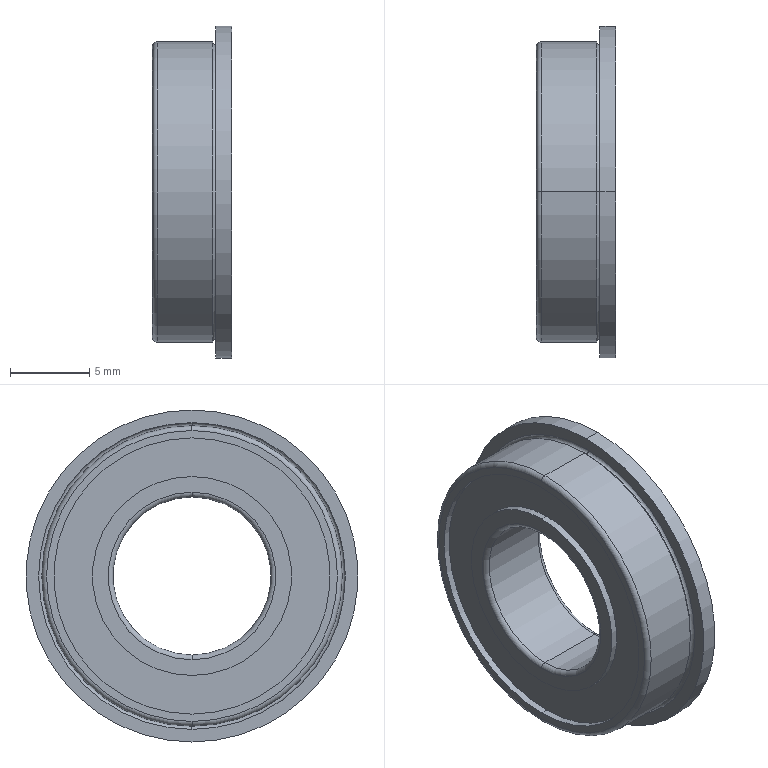Part | NX | features BREP 1 | 1 solid | 31 faces | box 5 x 21 x 21 mm | volume 978.232 mm3 | cylinder 14 | torus 10 | plane 7 | commonest cylinder face diameters 12.58 x4 17.47 x4 10 x2 19 x2 21 x2
STEP:
#1=CARTESIAN_POINT('',(0.,0.,9.3));
#2=VERTEX_POINT('',#1);
#3=CARTESIAN_POINT('',(-0.2,0.,9.5));
#4=VERTEX_POINT('',#3);
#5=CARTESIAN_POINT('',(0.,0.,9.5));
#6=DIRECTION('',(0.,-1.,0.));
#7=DIRECTION('',(0.,0.,-1.));
#8=AXIS2_PLACEMENT_3D('',#5,#6,#7);
#9=CIRCLE('',#8,0.2);
#10=EDGE_CURVE('',#2,#4,#9,.F.);
#11=ORIENTED_EDGE('',*,*,#10,.F.);
#12=CARTESIAN_POINT('',(0.,0.,-9.3));
#13=VERTEX_POINT('',#12);
#14=CARTESIAN_POINT('',(0.,0.,0.));
#15=DIRECTION('',(-1.,0.,0.));
#16=DIRECTION('',(0.,0.,1.));
#17=AXIS2_PLACEMENT_3D('',#14,#15,#16);
#18=CIRCLE('',#17,9.3);
#19=EDGE_CURVE('',#2,#13,#18,.T.);
#20=ORIENTED_EDGE('',*,*,#19,.T.);
#21=CARTESIAN_POINT('',(-0.2,0.,-9.5));
#22=VERTEX_POINT('',#21);
#23=CARTESIAN_POINT('',(0.,0.,-9.5));
#24=DIRECTION('',(0.,1.,0.));
#25=DIRECTION('',(0.,0.,1.));
#26=AXIS2_PLACEMENT_3D('',#23,#24,#25);
#27=CIRCLE('',#26,0.2);
#28=EDGE_CURVE('',#13,#22,#27,.F.);
#29=ORIENTED_EDGE('',*,*,#28,.T.);
#30=CARTESIAN_POINT('',(-0.2,0.,0.));
#31=DIRECTION('',(-1.,0.,0.));
#32=DIRECTION('',(0.,0.,1.));
#33=AXIS2_PLACEMENT_3D('',#30,#31,#32);
#34=CIRCLE('',#33,9.5);
#35=EDGE_CURVE('',#4,#22,#34,.T.);
#36=ORIENTED_EDGE('',*,*,#35,.F.);
#37=EDGE_LOOP('',(#11,#20,#29,#36));
#38=FACE_BOUND('',#37,.T.);
#39=CARTESIAN_POINT('',(0.,0.,0.));
#40=DIRECTION('',(-1.,0.,0.));
#41=DIRECTION('',(0.,0.,-1.));
#42=AXIS2_PLACEMENT_3D('',#39,#40,#41);
#43=TOROIDAL_SURFACE('',#42,9.5,0.2);
#44=ADVANCED_FACE('',(#38),#43,.F.);
#45=ORIENTED_EDGE('',*,*,#28,.F.);
#46=CARTESIAN_POINT('',(0.,0.,0.));
#47=DIRECTION('',(-1.,0.,0.));
#48=DIRECTION('',(0.,0.,1.));
#49=AXIS2_PLACEMENT_3D('',#46,#47,#48);
#50=CIRCLE('',#49,9.3);
#51=EDGE_CURVE('',#13,#2,#50,.T.);
#52=ORIENTED_EDGE('',*,*,#51,.T.);
#53=ORIENTED_EDGE('',*,*,#10,.T.);
#54=CARTESIAN_POINT('',(-0.2,0.,0.));
#55=DIRECTION('',(-1.,0.,0.));
#56=DIRECTION('',(0.,0.,1.));
#57=AXIS2_PLACEMENT_3D('',#54,#55,#56);
#58=CIRCLE('',#57,9.5);
#59=EDGE_CURVE('',#22,#4,#58,.T.);
#60=ORIENTED_EDGE('',*,*,#59,.F.);
#61=EDGE_LOOP('',(#45,#52,#53,#60));
#62=FACE_BOUND('',#61,.T.);
#63=CARTESIAN_POINT('',(0.,0.,0.));
#64=DIRECTION('',(-1.,0.,0.));
#65=DIRECTION('',(0.,0.,-1.));
#66=AXIS2_PLACEMENT_3D('',#63,#64,#65);
#67=TOROIDAL_SURFACE('',#66,9.5,0.2);
#68=ADVANCED_FACE('',(#62),#67,.F.);
#69=CARTESIAN_POINT('',(-4.,0.,9.2));
#70=VERTEX_POINT('',#69);
#71=CARTESIAN_POINT('',(-4.,0.,-9.2));
#72=VERTEX_POINT('',#71);
#73=CARTESIAN_POINT('',(-4.,0.,0.));
#74=DIRECTION('',(-1.,0.,0.));
#75=DIRECTION('',(0.,0.,-1.));
#76=AXIS2_PLACEMENT_3D('',#73,#74,#75);
#77=CIRCLE('',#76,9.2);
#78=EDGE_CURVE('',#70,#72,#77,.T.);
#79=ORIENTED_EDGE('',*,*,#78,.F.);
#80=CARTESIAN_POINT('',(-3.7,0.,9.5));
#81=VERTEX_POINT('',#80);
#82=CARTESIAN_POINT('',(-3.7,0.,9.2));
#83=DIRECTION('',(0.,1.,0.));
#84=DIRECTION('',(0.,0.,1.));
#85=AXIS2_PLACEMENT_3D('',#82,#83,#84);
#86=CIRCLE('',#85,0.3);
#87=EDGE_CURVE('',#81,#70,#86,.F.);
#88=ORIENTED_EDGE('',*,*,#87,.F.);
#89=CARTESIAN_POINT('',(-3.7,0.,-9.5));
#90=VERTEX_POINT('',#89);
#91=CARTESIAN_POINT('',(-3.7,0.,0.));
#92=DIRECTION('',(1.,0.,0.));
#93=DIRECTION('',(0.,0.,-1.));
#94=AXIS2_PLACEMENT_3D('',#91,#92,#93);
#95=CIRCLE('',#94,9.5);
#96=EDGE_CURVE('',#90,#81,#95,.T.);
#97=ORIENTED_EDGE('',*,*,#96,.F.);
#98=CARTESIAN_POINT('',(-3.7,0.,-9.2));
#99=DIRECTION('',(0.,-1.,0.));
#100=DIRECTION('',(0.,0.,-1.));
#101=AXIS2_PLACEMENT_3D('',#98,#99,#100);
#102=CIRCLE('',#101,0.3);
#103=EDGE_CURVE('',#90,#72,#102,.F.);
#104=ORIENTED_EDGE('',*,*,#103,.T.);
#105=EDGE_LOOP('',(#79,#88,#97,#104));
#106=FACE_BOUND('',#105,.T.);
#107=CARTESIAN_POINT('',(-3.7,0.,0.));
#108=DIRECTION('',(1.,0.,0.));
#109=DIRECTION('',(0.,0.,1.));
#110=AXIS2_PLACEMENT_3D('',#107,#108,#109);
#111=TOROIDAL_SURFACE('',#110,9.2,0.3);
#112=ADVANCED_FACE('',(#106),#111,.T.);
#113=CARTESIAN_POINT('',(-3.7,0.,5.));
#114=VERTEX_POINT('',#113);
#115=CARTESIAN_POINT('',(-3.7,0.,-5.));
#116=VERTEX_POINT('',#115);
#117=CARTESIAN_POINT('',(-3.7,0.,0.));
#118=DIRECTION('',(-1.,0.,0.));
#119=DIRECTION('',(0.,0.,-1.));
#120=AXIS2_PLACEMENT_3D('',#117,#118,#119);
#121=CIRCLE('',#120,5.);
#122=EDGE_CURVE('',#114,#116,#121,.T.);
#123=ORIENTED_EDGE('',*,*,#122,.F.);
#124=CARTESIAN_POINT('',(-4.,0.,5.3));
#125=VERTEX_POINT('',#124);
#126=CARTESIAN_POINT('',(-3.7,0.,5.3));
#127=DIRECTION('',(0.,1.,0.));
#128=DIRECTION('',(0.,0.,1.));
#129=AXIS2_PLACEMENT_3D('',#126,#127,#128);
#130=CIRCLE('',#129,0.3);
#131=EDGE_CURVE('',#125,#114,#130,.F.);
#132=ORIENTED_EDGE('',*,*,#131,.F.);
#133=CARTESIAN_POINT('',(-4.,0.,-5.3));
#134=VERTEX_POINT('',#133);
#135=CARTESIAN_POINT('',(-4.,0.,0.));
#136=DIRECTION('',(1.,0.,0.));
#137=DIRECTION('',(0.,0.,-1.));
#138=AXIS2_PLACEMENT_3D('',#135,#136,#137);
#139=CIRCLE('',#138,5.3);
#140=EDGE_CURVE('',#134,#125,#139,.T.);
#141=ORIENTED_EDGE('',*,*,#140,.F.);
#142=CARTESIAN_POINT('',(-3.7,0.,-5.3));
#143=DIRECTION('',(0.,-1.,0.));
#144=DIRECTION('',(0.,0.,-1.));
#145=AXIS2_PLACEMENT_3D('',#142,#143,#144);
#146=CIRCLE('',#145,0.3);
#147=EDGE_CURVE('',#134,#116,#146,.F.);
#148=ORIENTED_EDGE('',*,*,#147,.T.);
#149=EDGE_LOOP('',(#123,#132,#141,#148));
#150=FACE_BOUND('',#149,.T.);
#151=CARTESIAN_POINT('',(-3.7,0.,0.));
#152=DIRECTION('',(1.,0.,0.));
#153=DIRECTION('',(0.,0.,1.));
#154=AXIS2_PLACEMENT_3D('',#151,#152,#153);
#155=TOROIDAL_SURFACE('',#154,5.3,0.3);
#156=ADVANCED_FACE('',(#150),#155,.T.);
#157=CARTESIAN_POINT('',(0.7,0.,-5.));
#158=VERTEX_POINT('',#157);
#159=CARTESIAN_POINT('',(0.7,0.,5.));
#160=VERTEX_POINT('',#159);
#161=CARTESIAN_POINT('',(0.7,0.,0.));
#162=DIRECTION('',(1.,0.,0.));
#163=DIRECTION('',(0.,0.,1.));
#164=AXIS2_PLACEMENT_3D('',#161,#162,#163);
#165=CIRCLE('',#164,5.);
#166=EDGE_CURVE('',#158,#160,#165,.T.);
#167=ORIENTED_EDGE('',*,*,#166,.F.);
#168=CARTESIAN_POINT('',(1.,0.,-5.3));
#169=VERTEX_POINT('',#168);
#170=CARTESIAN_POINT('',(0.7,0.,-5.3));
#171=DIRECTION('',(0.,1.,0.));
#172=DIRECTION('',(0.,0.,1.));
#173=AXIS2_PLACEMENT_3D('',#170,#171,#172);
#174=CIRCLE('',#173,0.3);
#175=EDGE_CURVE('',#158,#169,#174,.T.);
#176=ORIENTED_EDGE('',*,*,#175,.T.);
#177=CARTESIAN_POINT('',(1.,0.,5.3));
#178=VERTEX_POINT('',#177);
#179=CARTESIAN_POINT('',(1.,0.,0.));
#180=DIRECTION('',(-1.,0.,0.));
#181=DIRECTION('',(0.,0.,1.));
#182=AXIS2_PLACEMENT_3D('',#179,#180,#181);
#183=CIRCLE('',#182,5.3);
#184=EDGE_CURVE('',#178,#169,#183,.T.);
#185=ORIENTED_EDGE('',*,*,#184,.F.);
#186=CARTESIAN_POINT('',(0.7,0.,5.3));
#187=DIRECTION('',(0.,-1.,0.));
#188=DIRECTION('',(0.,0.,-1.));
#189=AXIS2_PLACEMENT_3D('',#186,#187,#188);
#190=CIRCLE('',#189,0.3);
#191=EDGE_CURVE('',#160,#178,#190,.T.);
#192=ORIENTED_EDGE('',*,*,#191,.F.);
#193=EDGE_LOOP('',(#167,#176,#185,#192));
#194=FACE_BOUND('',#193,.T.);
#195=CARTESIAN_POINT('',(0.7,0.,0.));
#196=DIRECTION('',(-1.,0.,0.));
#197=DIRECTION('',(0.,0.,-1.));
#198=AXIS2_PLACEMENT_3D('',#195,#196,#197);
#199=TOROIDAL_SURFACE('',#198,5.3,0.3);
#200=ADVANCED_FACE('',(#194),#199,.T.);
#201=CARTESIAN_POINT('',(1.,0.,-8.735));
#202=VERTEX_POINT('',#201);
#203=CARTESIAN_POINT('',(1.,0.,8.735));
#204=VERTEX_POINT('',#203);
#205=CARTESIAN_POINT('',(1.,0.,0.));
#206=DIRECTION('',(-1.,0.,0.));
#207=DIRECTION('',(0.,0.,1.));
#208=AXIS2_PLACEMENT_3D('',#205,#206,#207);
#209=CIRCLE('',#208,8.735);
#210=EDGE_CURVE('',#202,#204,#209,.T.);
#211=ORIENTED_EDGE('',*,*,#210,.F.);
#212=CARTESIAN_POINT('',(0.56,0.,-8.735));
#213=VERTEX_POINT('',#212);
#214=CARTESIAN_POINT('',(-4.,0.,-8.735));
#215=DIRECTION('',(-1.,0.,0.));
#216=VECTOR('',#215,1000.);
#217=LINE('',#214,#216);
#218=EDGE_CURVE('',#202,#213,#217,.T.);
#219=ORIENTED_EDGE('',*,*,#218,.T.);
#220=CARTESIAN_POINT('',(0.56,0.,8.735));
#221=VERTEX_POINT('',#220);
#222=CARTESIAN_POINT('',(0.56,0.,0.));
#223=DIRECTION('',(-1.,0.,0.));
#224=DIRECTION('',(0.,0.,1.));
#225=AXIS2_PLACEMENT_3D('',#222,#223,#224);
#226=CIRCLE('',#225,8.735);
#227=EDGE_CURVE('',#213,#221,#226,.T.);
#228=ORIENTED_EDGE('',*,*,#227,.T.);
#229=CARTESIAN_POINT('',(-4.,0.,8.735));
#230=DIRECTION('',(-1.,0.,0.));
#231=VECTOR('',#230,1000.);
#232=LINE('',#229,#231);
#233=EDGE_CURVE('',#204,#221,#232,.T.);
#234=ORIENTED_EDGE('',*,*,#233,.F.);
#235=EDGE_LOOP('',(#211,#219,#228,#234));
#236=FACE_BOUND('',#235,.T.);
#237=CARTESIAN_POINT('',(-4.,0.,0.));
#238=DIRECTION('',(-1.,0.,0.));
#239=DIRECTION('',(0.,0.,-1.));
#240=AXIS2_PLACEMENT_3D('',#237,#238,#239);
#241=CYLINDRICAL_SURFACE('',#240,8.735);
#242=ADVANCED_FACE('',(#236),#241,.F.);
#243=CARTESIAN_POINT('',(1.,0.,6.29));
#244=VERTEX_POINT('',#243);
#245=CARTESIAN_POINT('',(1.,0.,-6.29));
#246=VERTEX_POINT('',#245);
#247=CARTESIAN_POINT('',(1.,0.,0.));
#248=DIRECTION('',(-1.,0.,0.));
#249=DIRECTION('',(0.,0.,1.));
#250=AXIS2_PLACEMENT_3D('',#247,#248,#249);
#251=CIRCLE('',#250,6.29);
#252=EDGE_CURVE('',#244,#246,#251,.T.);
#253=ORIENTED_EDGE('',*,*,#252,.T.);
#254=CARTESIAN_POINT('',(0.56,0.,-6.29));
#255=VERTEX_POINT('',#254);
#256=CARTESIAN_POINT('',(-4.,0.,-6.29));
#257=DIRECTION('',(-1.,0.,0.));
#258=VECTOR('',#257,1000.);
#259=LINE('',#256,#258);
#260=EDGE_CURVE('',#246,#255,#259,.T.);
#261=ORIENTED_EDGE('',*,*,#260,.T.);
#262=CARTESIAN_POINT('',(0.56,0.,6.29));
#263=VERTEX_POINT('',#262);
#264=CARTESIAN_POINT('',(0.56,0.,0.));
#265=DIRECTION('',(-1.,0.,0.));
#266=DIRECTION('',(0.,0.,1.));
#267=AXIS2_PLACEMENT_3D('',#264,#265,#266);
#268=CIRCLE('',#267,6.29);
#269=EDGE_CURVE('',#263,#255,#268,.T.);
#270=ORIENTED_EDGE('',*,*,#269,.F.);
#271=CARTESIAN_POINT('',(-4.,0.,6.29));
#272=DIRECTION('',(-1.,0.,0.));
#273=VECTOR('',#272,1000.);
#274=LINE('',#271,#273);
#275=EDGE_CURVE('',#244,#263,#274,.T.);
#276=ORIENTED_EDGE('',*,*,#275,.F.);
#277=EDGE_LOOP('',(#253,#261,#270,#276));
#278=FACE_BOUND('',#277,.T.);
#279=CARTESIAN_POINT('',(-4.,0.,0.));
#280=DIRECTION('',(-1.,0.,0.));
#281=DIRECTION('',(0.,0.,-1.));
#282=AXIS2_PLACEMENT_3D('',#279,#280,#281);
#283=CYLINDRICAL_SURFACE('',#282,6.29);
#284=ADVANCED_FACE('',(#278),#283,.T.);
#285=CARTESIAN_POINT('',(0.7,0.,0.));
#286=DIRECTION('',(1.,0.,0.));
#287=DIRECTION('',(0.,0.,1.));
#288=AXIS2_PLACEMENT_3D('',#285,#286,#287);
#289=CIRCLE('',#288,5.);
#290=EDGE_CURVE('',#160,#158,#289,.T.);
#291=ORIENTED_EDGE('',*,*,#290,.T.);
#292=CARTESIAN_POINT('',(-4.,0.,-5.));
#293=DIRECTION('',(-1.,0.,0.));
#294=VECTOR('',#293,1000.);
#295=LINE('',#292,#294);
#296=EDGE_CURVE('',#158,#116,#295,.T.);
#297=ORIENTED_EDGE('',*,*,#296,.T.);
#298=CARTESIAN_POINT('',(-3.7,0.,0.));
#299=DIRECTION('',(-1.,0.,0.));
#300=DIRECTION('',(0.,0.,-1.));
#301=AXIS2_PLACEMENT_3D('',#298,#299,#300);
#302=CIRCLE('',#301,5.);
#303=EDGE_CURVE('',#116,#114,#302,.T.);
#304=ORIENTED_EDGE('',*,*,#303,.T.);
#305=CARTESIAN_POINT('',(-4.,0.,5.));
#306=DIRECTION('',(-1.,0.,0.));
#307=VECTOR('',#306,1000.);
#308=LINE('',#305,#307);
#309=EDGE_CURVE('',#160,#114,#308,.T.);
#310=ORIENTED_EDGE('',*,*,#309,.F.);
#311=EDGE_LOOP('',(#291,#297,#304,#310));
#312=FACE_BOUND('',#311,.T.);
#313=CARTESIAN_POINT('',(-4.,0.,0.));
#314=DIRECTION('',(-1.,0.,0.));
#315=DIRECTION('',(0.,0.,-1.));
#316=AXIS2_PLACEMENT_3D('',#313,#314,#315);
#317=CYLINDRICAL_SURFACE('',#316,5.);
#318=ADVANCED_FACE('',(#312),#317,.F.);
#319=CARTESIAN_POINT('',(-3.56,0.,6.29));
#320=VERTEX_POINT('',#319);
#321=CARTESIAN_POINT('',(-3.56,0.,-6.29));
#322=VERTEX_POINT('',#321);
#323=CARTESIAN_POINT('',(-3.56,0.,0.));
#324=DIRECTION('',(-1.,0.,0.));
#325=DIRECTION('',(0.,0.,1.));
#326=AXIS2_PLACEMENT_3D('',#323,#324,#325);
#327=CIRCLE('',#326,6.29);
#328=EDGE_CURVE('',#320,#322,#327,.T.);
#329=ORIENTED_EDGE('',*,*,#328,.T.);
#330=CARTESIAN_POINT('',(-4.,0.,-6.29));
#331=VERTEX_POINT('',#330);
#332=CARTESIAN_POINT('',(-4.,0.,-6.29));
#333=DIRECTION('',(-1.,0.,0.));
#334=VECTOR('',#333,1000.);
#335=LINE('',#332,#334);
#336=EDGE_CURVE('',#322,#331,#335,.T.);
#337=ORIENTED_EDGE('',*,*,#336,.T.);
#338=CARTESIAN_POINT('',(-4.,0.,6.29));
#339=VERTEX_POINT('',#338);
#340=CARTESIAN_POINT('',(-4.,0.,0.));
#341=DIRECTION('',(-1.,0.,0.));
#342=DIRECTION('',(0.,0.,1.));
#343=AXIS2_PLACEMENT_3D('',#340,#341,#342);
#344=CIRCLE('',#343,6.29);
#345=EDGE_CURVE('',#339,#331,#344,.T.);
#346=ORIENTED_EDGE('',*,*,#345,.F.);
#347=CARTESIAN_POINT('',(-4.,0.,6.29));
#348=DIRECTION('',(-1.,0.,0.));
#349=VECTOR('',#348,1000.);
#350=LINE('',#347,#349);
#351=EDGE_CURVE('',#320,#339,#350,.T.);
#352=ORIENTED_EDGE('',*,*,#351,.F.);
#353=EDGE_LOOP('',(#329,#337,#346,#352));
#354=FACE_BOUND('',#353,.T.);
#355=CARTESIAN_POINT('',(-4.,0.,0.));
#356=DIRECTION('',(-1.,0.,0.));
#357=DIRECTION('',(0.,0.,-1.));
#358=AXIS2_PLACEMENT_3D('',#355,#356,#357);
#359=CYLINDRICAL_SURFACE('',#358,6.29);
#360=ADVANCED_FACE('',(#354),#359,.T.);
#361=CARTESIAN_POINT('',(-3.56,0.,-8.735));
#362=VERTEX_POINT('',#361);
#363=CARTESIAN_POINT('',(-3.56,0.,8.735));
#364=VERTEX_POINT('',#363);
#365=CARTESIAN_POINT('',(-3.56,0.,0.));
#366=DIRECTION('',(-1.,0.,0.));
#367=DIRECTION('',(0.,0.,1.));
#368=AXIS2_PLACEMENT_3D('',#365,#366,#367);
#369=CIRCLE('',#368,8.735);
#370=EDGE_CURVE('',#362,#364,#369,.T.);
#371=ORIENTED_EDGE('',*,*,#370,.F.);
#372=CARTESIAN_POINT('',(-4.,0.,-8.735));
#373=VERTEX_POINT('',#372);
#374=CARTESIAN_POINT('',(-4.,0.,-8.735));
#375=DIRECTION('',(-1.,0.,0.));
#376=VECTOR('',#375,1000.);
#377=LINE('',#374,#376);
#378=EDGE_CURVE('',#362,#373,#377,.T.);
#379=ORIENTED_EDGE('',*,*,#378,.T.);
#380=CARTESIAN_POINT('',(-4.,0.,8.735));
#381=VERTEX_POINT('',#380);
#382=CARTESIAN_POINT('',(-4.,0.,0.));
#383=DIRECTION('',(-1.,0.,0.));
#384=DIRECTION('',(0.,0.,1.));
#385=AXIS2_PLACEMENT_3D('',#382,#383,#384);
#386=CIRCLE('',#385,8.735);
#387=EDGE_CURVE('',#373,#381,#386,.T.);
#388=ORIENTED_EDGE('',*,*,#387,.T.);
#389=CARTESIAN_POINT('',(-4.,0.,8.735));
#390=DIRECTION('',(-1.,0.,0.));
#391=VECTOR('',#390,1000.);
#392=LINE('',#389,#391);
#393=EDGE_CURVE('',#364,#381,#392,.T.);
#394=ORIENTED_EDGE('',*,*,#393,.F.);
#395=EDGE_LOOP('',(#371,#379,#388,#394));
#396=FACE_BOUND('',#395,.T.);
#397=CARTESIAN_POINT('',(-4.,0.,0.));
#398=DIRECTION('',(-1.,0.,0.));
#399=DIRECTION('',(0.,0.,-1.));
#400=AXIS2_PLACEMENT_3D('',#397,#398,#399);
#401=CYLINDRICAL_SURFACE('',#400,8.735);
#402=ADVANCED_FACE('',(#396),#401,.F.);
#403=ORIENTED_EDGE('',*,*,#35,.T.);
#404=CARTESIAN_POINT('',(-4.,0.,-9.5));
#405=DIRECTION('',(-1.,0.,0.));
#406=VECTOR('',#405,1000.);
#407=LINE('',#404,#406);
#408=EDGE_CURVE('',#22,#90,#407,.T.);
#409=ORIENTED_EDGE('',*,*,#408,.T.);
#410=ORIENTED_EDGE('',*,*,#96,.T.);
#411=CARTESIAN_POINT('',(-4.,0.,9.5));
#412=DIRECTION('',(-1.,0.,0.));
#413=VECTOR('',#412,1000.);
#414=LINE('',#411,#413);
#415=EDGE_CURVE('',#4,#81,#414,.T.);
#416=ORIENTED_EDGE('',*,*,#415,.F.);
#417=EDGE_LOOP('',(#403,#409,#410,#416));
#418=FACE_BOUND('',#417,.T.);
#419=CARTESIAN_POINT('',(-4.,0.,0.));
#420=DIRECTION('',(-1.,0.,0.));
#421=DIRECTION('',(0.,0.,-1.));
#422=AXIS2_PLACEMENT_3D('',#419,#420,#421);
#423=CYLINDRICAL_SURFACE('',#422,9.5);
#424=ADVANCED_FACE('',(#418),#423,.T.);
#425=ORIENTED_EDGE('',*,*,#51,.F.);
#426=CARTESIAN_POINT('',(0.,0.,-9.7));
#427=VERTEX_POINT('',#426);
#428=CARTESIAN_POINT('',(0.,0.,-9.5));
#429=DIRECTION('',(0.,1.,0.));
#430=DIRECTION('',(0.,0.,1.));
#431=AXIS2_PLACEMENT_3D('',#428,#429,#430);
#432=CIRCLE('',#431,0.2);
#433=EDGE_CURVE('',#13,#427,#432,.T.);
#434=ORIENTED_EDGE('',*,*,#433,.T.);
#435=CARTESIAN_POINT('',(0.,0.,9.7));
#436=VERTEX_POINT('',#435);
#437=CARTESIAN_POINT('',(0.,0.,0.));
#438=DIRECTION('',(-1.,0.,0.));
#439=DIRECTION('',(0.,0.,1.));
#440=AXIS2_PLACEMENT_3D('',#437,#438,#439);
#441=CIRCLE('',#440,9.7);
#442=EDGE_CURVE('',#427,#436,#441,.T.);
#443=ORIENTED_EDGE('',*,*,#442,.T.);
#444=CARTESIAN_POINT('',(0.,0.,9.5));
#445=DIRECTION('',(0.,-1.,0.));
#446=DIRECTION('',(0.,0.,-1.));
#447=AXIS2_PLACEMENT_3D('',#444,#445,#446);
#448=CIRCLE('',#447,0.2);
#449=EDGE_CURVE('',#2,#436,#448,.T.);
#450=ORIENTED_EDGE('',*,*,#449,.F.);
#451=EDGE_LOOP('',(#425,#434,#443,#450));
#452=FACE_BOUND('',#451,.T.);
#453=CARTESIAN_POINT('',(0.,0.,0.));
#454=DIRECTION('',(-1.,0.,0.));
#455=DIRECTION('',(0.,0.,-1.));
#456=AXIS2_PLACEMENT_3D('',#453,#454,#455);
#457=TOROIDAL_SURFACE('',#456,9.5,0.2);
#458=ADVANCED_FACE('',(#452),#457,.F.);
#459=CARTESIAN_POINT('',(1.,0.,10.5));
#460=VERTEX_POINT('',#459);
#461=CARTESIAN_POINT('',(1.,0.,-10.5));
#462=VERTEX_POINT('',#461);
#463=CARTESIAN_POINT('',(1.,0.,0.));
#464=DIRECTION('',(-1.,0.,0.));
#465=DIRECTION('',(0.,0.,1.));
#466=AXIS2_PLACEMENT_3D('',#463,#464,#465);
#467=CIRCLE('',#466,10.5);
#468=EDGE_CURVE('',#460,#462,#467,.T.);
#469=ORIENTED_EDGE('',*,*,#468,.T.);
#470=CARTESIAN_POINT('',(0.,0.,-10.5));
#471=VERTEX_POINT('',#470);
#472=CARTESIAN_POINT('',(-4.,0.,-10.5));
#473=DIRECTION('',(-1.,0.,0.));
#474=VECTOR('',#473,1000.);
#475=LINE('',#472,#474);
#476=EDGE_CURVE('',#462,#471,#475,.T.);
#477=ORIENTED_EDGE('',*,*,#476,.T.);
#478=CARTESIAN_POINT('',(0.,0.,10.5));
#479=VERTEX_POINT('',#478);
#480=CARTESIAN_POINT('',(0.,0.,0.));
#481=DIRECTION('',(-1.,0.,0.));
#482=DIRECTION('',(0.,0.,1.));
#483=AXIS2_PLACEMENT_3D('',#480,#481,#482);
#484=CIRCLE('',#483,10.5);
#485=EDGE_CURVE('',#479,#471,#484,.T.);
#486=ORIENTED_EDGE('',*,*,#485,.F.);
#487=CARTESIAN_POINT('',(-4.,0.,10.5));
#488=DIRECTION('',(-1.,0.,0.));
#489=VECTOR('',#488,1000.);
#490=LINE('',#487,#489);
#491=EDGE_CURVE('',#460,#479,#490,.T.);
#492=ORIENTED_EDGE('',*,*,#491,.F.);
#493=EDGE_LOOP('',(#469,#477,#486,#492));
#494=FACE_BOUND('',#493,.T.);
#495=CARTESIAN_POINT('',(-4.,0.,0.));
#496=DIRECTION('',(-1.,0.,0.));
#497=DIRECTION('',(0.,0.,-1.));
#498=AXIS2_PLACEMENT_3D('',#495,#496,#497);
#499=CYLINDRICAL_SURFACE('',#498,10.5);
#500=ADVANCED_FACE('',(#494),#499,.T.);
#501=ORIENTED_EDGE('',*,*,#476,.F.);
#502=CARTESIAN_POINT('',(1.,0.,0.));
#503=DIRECTION('',(-1.,0.,0.));
#504=DIRECTION('',(0.,0.,1.));
#505=AXIS2_PLACEMENT_3D('',#502,#503,#504);
#506=CIRCLE('',#505,10.5);
#507=EDGE_CURVE('',#462,#460,#506,.T.);
#508=ORIENTED_EDGE('',*,*,#507,.T.);
#509=ORIENTED_EDGE('',*,*,#491,.T.);
#510=CARTESIAN_POINT('',(0.,0.,0.));
#511=DIRECTION('',(-1.,0.,0.));
#512=DIRECTION('',(0.,0.,1.));
#513=AXIS2_PLACEMENT_3D('',#510,#511,#512);
#514=CIRCLE('',#513,10.5);
#515=EDGE_CURVE('',#471,#479,#514,.T.);
#516=ORIENTED_EDGE('',*,*,#515,.F.);
#517=EDGE_LOOP('',(#501,#508,#509,#516));
#518=FACE_BOUND('',#517,.T.);
#519=CARTESIAN_POINT('',(-4.,0.,0.));
#520=DIRECTION('',(-1.,0.,0.));
#521=DIRECTION('',(0.,0.,-1.));
#522=AXIS2_PLACEMENT_3D('',#519,#520,#521);
#523=CYLINDRICAL_SURFACE('',#522,10.5);
#524=ADVANCED_FACE('',(#518),#523,.T.);
#525=ORIENTED_EDGE('',*,*,#485,.T.);
#526=ORIENTED_EDGE('',*,*,#515,.T.);
#527=EDGE_LOOP('',(#525,#526));
#528=FACE_BOUND('',#527,.T.);
#529=CARTESIAN_POINT('',(0.,0.,0.));
#530=DIRECTION('',(-1.,0.,0.));
#531=DIRECTION('',(0.,0.,1.));
#532=AXIS2_PLACEMENT_3D('',#529,#530,#531);
#533=CIRCLE('',#532,9.7);
#534=EDGE_CURVE('',#436,#427,#533,.T.);
#535=ORIENTED_EDGE('',*,*,#534,.F.);
#536=ORIENTED_EDGE('',*,*,#442,.F.);
#537=EDGE_LOOP('',(#535,#536));
#538=FACE_BOUND('',#537,.T.);
#539=CARTESIAN_POINT('',(0.,9.7,0.));
#540=DIRECTION('',(1.,0.,0.));
#541=DIRECTION('',(0.,-1.,0.));
#542=AXIS2_PLACEMENT_3D('',#539,#540,#541);
#543=PLANE('',#542);
#544=ADVANCED_FACE('',(#528,#538),#543,.F.);
#545=ORIENTED_EDGE('',*,*,#19,.F.);
#546=ORIENTED_EDGE('',*,*,#449,.T.);
#547=ORIENTED_EDGE('',*,*,#534,.T.);
#548=ORIENTED_EDGE('',*,*,#433,.F.);
#549=EDGE_LOOP('',(#545,#546,#547,#548));
#550=FACE_BOUND('',#549,.T.);
#551=CARTESIAN_POINT('',(0.,0.,0.));
#552=DIRECTION('',(-1.,0.,0.));
#553=DIRECTION('',(0.,0.,-1.));
#554=AXIS2_PLACEMENT_3D('',#551,#552,#553);
#555=TOROIDAL_SURFACE('',#554,9.5,0.2);
#556=ADVANCED_FACE('',(#550),#555,.F.);
#557=ORIENTED_EDGE('',*,*,#408,.F.);
#558=ORIENTED_EDGE('',*,*,#59,.T.);
#559=ORIENTED_EDGE('',*,*,#415,.T.);
#560=CARTESIAN_POINT('',(-3.7,0.,0.));
#561=DIRECTION('',(1.,0.,0.));
#562=DIRECTION('',(0.,0.,-1.));
#563=AXIS2_PLACEMENT_3D('',#560,#561,#562);
#564=CIRCLE('',#563,9.5);
#565=EDGE_CURVE('',#81,#90,#564,.T.);
#566=ORIENTED_EDGE('',*,*,#565,.T.);
#567=EDGE_LOOP('',(#557,#558,#559,#566));
#568=FACE_BOUND('',#567,.T.);
#569=CARTESIAN_POINT('',(-4.,0.,0.));
#570=DIRECTION('',(-1.,0.,0.));
#571=DIRECTION('',(0.,0.,-1.));
#572=AXIS2_PLACEMENT_3D('',#569,#570,#571);
#573=CYLINDRICAL_SURFACE('',#572,9.5);
#574=ADVANCED_FACE('',(#568),#573,.T.);
#575=CARTESIAN_POINT('',(-4.,0.,0.));
#576=DIRECTION('',(-1.,0.,0.));
#577=DIRECTION('',(0.,0.,-1.));
#578=AXIS2_PLACEMENT_3D('',#575,#576,#577);
#579=CIRCLE('',#578,9.2);
#580=EDGE_CURVE('',#72,#70,#579,.T.);
#581=ORIENTED_EDGE('',*,*,#580,.T.);
#582=ORIENTED_EDGE('',*,*,#78,.T.);
#583=EDGE_LOOP('',(#581,#582));
#584=FACE_BOUND('',#583,.T.);
#585=CARTESIAN_POINT('',(-4.,0.,0.));
#586=DIRECTION('',(-1.,0.,0.));
#587=DIRECTION('',(0.,0.,1.));
#588=AXIS2_PLACEMENT_3D('',#585,#586,#587);
#589=CIRCLE('',#588,8.735);
#590=EDGE_CURVE('',#381,#373,#589,.T.);
#591=ORIENTED_EDGE('',*,*,#590,.F.);
#592=ORIENTED_EDGE('',*,*,#387,.F.);
#593=EDGE_LOOP('',(#591,#592));
#594=FACE_BOUND('',#593,.T.);
#595=CARTESIAN_POINT('',(-4.,8.735,0.));
#596=DIRECTION('',(1.,0.,0.));
#597=DIRECTION('',(0.,-1.,0.));
#598=AXIS2_PLACEMENT_3D('',#595,#596,#597);
#599=PLANE('',#598);
#600=ADVANCED_FACE('',(#584,#594),#599,.F.);
#601=ORIENTED_EDGE('',*,*,#378,.F.);
#602=CARTESIAN_POINT('',(-3.56,0.,0.));
#603=DIRECTION('',(-1.,0.,0.));
#604=DIRECTION('',(0.,0.,1.));
#605=AXIS2_PLACEMENT_3D('',#602,#603,#604);
#606=CIRCLE('',#605,8.735);
#607=EDGE_CURVE('',#364,#362,#606,.T.);
#608=ORIENTED_EDGE('',*,*,#607,.F.);
#609=ORIENTED_EDGE('',*,*,#393,.T.);
#610=ORIENTED_EDGE('',*,*,#590,.T.);
#611=EDGE_LOOP('',(#601,#608,#609,#610));
#612=FACE_BOUND('',#611,.T.);
#613=CARTESIAN_POINT('',(-4.,0.,0.));
#614=DIRECTION('',(-1.,0.,0.));
#615=DIRECTION('',(0.,0.,-1.));
#616=AXIS2_PLACEMENT_3D('',#613,#614,#615);
#617=CYLINDRICAL_SURFACE('',#616,8.735);
#618=ADVANCED_FACE('',(#612),#617,.F.);
#619=ORIENTED_EDGE('',*,*,#607,.T.);
#620=ORIENTED_EDGE('',*,*,#370,.T.);
#621=EDGE_LOOP('',(#619,#620));
#622=FACE_BOUND('',#621,.T.);
#623=ORIENTED_EDGE('',*,*,#328,.F.);
#624=CARTESIAN_POINT('',(-3.56,0.,0.));
#625=DIRECTION('',(-1.,0.,0.));
#626=DIRECTION('',(0.,0.,1.));
#627=AXIS2_PLACEMENT_3D('',#624,#625,#626);
#628=CIRCLE('',#627,6.29);
#629=EDGE_CURVE('',#322,#320,#628,.T.);
#630=ORIENTED_EDGE('',*,*,#629,.F.);
#631=EDGE_LOOP('',(#623,#630));
#632=FACE_BOUND('',#631,.T.);
#633=CARTESIAN_POINT('',(-3.56,8.735,0.));
#634=DIRECTION('',(1.,0.,0.));
#635=DIRECTION('',(0.,-1.,0.));
#636=AXIS2_PLACEMENT_3D('',#633,#634,#635);
#637=PLANE('',#636);
#638=ADVANCED_FACE('',(#622,#632),#637,.F.);
#639=ORIENTED_EDGE('',*,*,#336,.F.);
#640=ORIENTED_EDGE('',*,*,#629,.T.);
#641=ORIENTED_EDGE('',*,*,#351,.T.);
#642=CARTESIAN_POINT('',(-4.,0.,0.));
#643=DIRECTION('',(-1.,0.,0.));
#644=DIRECTION('',(0.,0.,1.));
#645=AXIS2_PLACEMENT_3D('',#642,#643,#644);
#646=CIRCLE('',#645,6.29);
#647=EDGE_CURVE('',#331,#339,#646,.T.);
#648=ORIENTED_EDGE('',*,*,#647,.F.);
#649=EDGE_LOOP('',(#639,#640,#641,#648));
#650=FACE_BOUND('',#649,.T.);
#651=CARTESIAN_POINT('',(-4.,0.,0.));
#652=DIRECTION('',(-1.,0.,0.));
#653=DIRECTION('',(0.,0.,-1.));
#654=AXIS2_PLACEMENT_3D('',#651,#652,#653);
#655=CYLINDRICAL_SURFACE('',#654,6.29);
#656=ADVANCED_FACE('',(#650),#655,.T.);
#657=ORIENTED_EDGE('',*,*,#345,.T.);
#658=ORIENTED_EDGE('',*,*,#647,.T.);
#659=EDGE_LOOP('',(#657,#658));
#660=FACE_BOUND('',#659,.T.);
#661=ORIENTED_EDGE('',*,*,#140,.T.);
#662=CARTESIAN_POINT('',(-4.,0.,0.));
#663=DIRECTION('',(1.,0.,0.));
#664=DIRECTION('',(0.,0.,-1.));
#665=AXIS2_PLACEMENT_3D('',#662,#663,#664);
#666=CIRCLE('',#665,5.3);
#667=EDGE_CURVE('',#125,#134,#666,.T.);
#668=ORIENTED_EDGE('',*,*,#667,.T.);
#669=EDGE_LOOP('',(#661,#668));
#670=FACE_BOUND('',#669,.T.);
#671=CARTESIAN_POINT('',(-4.,5.,0.));
#672=DIRECTION('',(1.,0.,0.));
#673=DIRECTION('',(0.,-1.,0.));
#674=AXIS2_PLACEMENT_3D('',#671,#672,#673);
#675=PLANE('',#674);
#676=ADVANCED_FACE('',(#660,#670),#675,.F.);
#677=ORIENTED_EDGE('',*,*,#296,.F.);
#678=ORIENTED_EDGE('',*,*,#166,.T.);
#679=ORIENTED_EDGE('',*,*,#309,.T.);
#680=ORIENTED_EDGE('',*,*,#122,.T.);
#681=EDGE_LOOP('',(#677,#678,#679,#680));
#682=FACE_BOUND('',#681,.T.);
#683=CARTESIAN_POINT('',(-4.,0.,0.));
#684=DIRECTION('',(-1.,0.,0.));
#685=DIRECTION('',(0.,0.,-1.));
#686=AXIS2_PLACEMENT_3D('',#683,#684,#685);
#687=CYLINDRICAL_SURFACE('',#686,5.);
#688=ADVANCED_FACE('',(#682),#687,.F.);
#689=ORIENTED_EDGE('',*,*,#252,.F.);
#690=CARTESIAN_POINT('',(1.,0.,0.));
#691=DIRECTION('',(-1.,0.,0.));
#692=DIRECTION('',(0.,0.,1.));
#693=AXIS2_PLACEMENT_3D('',#690,#691,#692);
#694=CIRCLE('',#693,6.29);
#695=EDGE_CURVE('',#246,#244,#694,.T.);
#696=ORIENTED_EDGE('',*,*,#695,.F.);
#697=EDGE_LOOP('',(#689,#696));
#698=FACE_BOUND('',#697,.T.);
#699=ORIENTED_EDGE('',*,*,#184,.T.);
#700=CARTESIAN_POINT('',(1.,0.,0.));
#701=DIRECTION('',(-1.,0.,0.));
#702=DIRECTION('',(0.,0.,1.));
#703=AXIS2_PLACEMENT_3D('',#700,#701,#702);
#704=CIRCLE('',#703,5.3);
#705=EDGE_CURVE('',#169,#178,#704,.T.);
#706=ORIENTED_EDGE('',*,*,#705,.T.);
#707=EDGE_LOOP('',(#699,#706));
#708=FACE_BOUND('',#707,.T.);
#709=CARTESIAN_POINT('',(1.,6.29,0.));
#710=DIRECTION('',(-1.,0.,0.));
#711=DIRECTION('',(0.,0.,-1.));
#712=AXIS2_PLACEMENT_3D('',#709,#710,#711);
#713=PLANE('',#712);
#714=ADVANCED_FACE('',(#698,#708),#713,.F.);
#715=ORIENTED_EDGE('',*,*,#260,.F.);
#716=ORIENTED_EDGE('',*,*,#695,.T.);
#717=ORIENTED_EDGE('',*,*,#275,.T.);
#718=CARTESIAN_POINT('',(0.56,0.,0.));
#719=DIRECTION('',(-1.,0.,0.));
#720=DIRECTION('',(0.,0.,1.));
#721=AXIS2_PLACEMENT_3D('',#718,#719,#720);
#722=CIRCLE('',#721,6.29);
#723=EDGE_CURVE('',#255,#263,#722,.T.);
#724=ORIENTED_EDGE('',*,*,#723,.F.);
#725=EDGE_LOOP('',(#715,#716,#717,#724));
#726=FACE_BOUND('',#725,.T.);
#727=CARTESIAN_POINT('',(-4.,0.,0.));
#728=DIRECTION('',(-1.,0.,0.));
#729=DIRECTION('',(0.,0.,-1.));
#730=AXIS2_PLACEMENT_3D('',#727,#728,#729);
#731=CYLINDRICAL_SURFACE('',#730,6.29);
#732=ADVANCED_FACE('',(#726),#731,.T.);
#733=CARTESIAN_POINT('',(0.56,0.,0.));
#734=DIRECTION('',(-1.,0.,0.));
#735=DIRECTION('',(0.,0.,1.));
#736=AXIS2_PLACEMENT_3D('',#733,#734,#735);
#737=CIRCLE('',#736,8.735);
#738=EDGE_CURVE('',#221,#213,#737,.T.);
#739=ORIENTED_EDGE('',*,*,#738,.F.);
#740=ORIENTED_EDGE('',*,*,#227,.F.);
#741=EDGE_LOOP('',(#739,#740));
#742=FACE_BOUND('',#741,.T.);
#743=ORIENTED_EDGE('',*,*,#269,.T.);
#744=ORIENTED_EDGE('',*,*,#723,.T.);
#745=EDGE_LOOP('',(#743,#744));
#746=FACE_BOUND('',#745,.T.);
#747=CARTESIAN_POINT('',(0.56,8.735,0.));
#748=DIRECTION('',(-1.,0.,0.));
#749=DIRECTION('',(0.,0.,-1.));
#750=AXIS2_PLACEMENT_3D('',#747,#748,#749);
#751=PLANE('',#750);
#752=ADVANCED_FACE('',(#742,#746),#751,.F.);
#753=ORIENTED_EDGE('',*,*,#218,.F.);
#754=CARTESIAN_POINT('',(1.,0.,0.));
#755=DIRECTION('',(-1.,0.,0.));
#756=DIRECTION('',(0.,0.,1.));
#757=AXIS2_PLACEMENT_3D('',#754,#755,#756);
#758=CIRCLE('',#757,8.735);
#759=EDGE_CURVE('',#204,#202,#758,.T.);
#760=ORIENTED_EDGE('',*,*,#759,.F.);
#761=ORIENTED_EDGE('',*,*,#233,.T.);
#762=ORIENTED_EDGE('',*,*,#738,.T.);
#763=EDGE_LOOP('',(#753,#760,#761,#762));
#764=FACE_BOUND('',#763,.T.);
#765=CARTESIAN_POINT('',(-4.,0.,0.));
#766=DIRECTION('',(-1.,0.,0.));
#767=DIRECTION('',(0.,0.,-1.));
#768=AXIS2_PLACEMENT_3D('',#765,#766,#767);
#769=CYLINDRICAL_SURFACE('',#768,8.735);
#770=ADVANCED_FACE('',(#764),#769,.F.);
#771=ORIENTED_EDGE('',*,*,#468,.F.);
#772=ORIENTED_EDGE('',*,*,#507,.F.);
#773=EDGE_LOOP('',(#771,#772));
#774=FACE_BOUND('',#773,.T.);
#775=ORIENTED_EDGE('',*,*,#759,.T.);
#776=ORIENTED_EDGE('',*,*,#210,.T.);
#777=EDGE_LOOP('',(#775,#776));
#778=FACE_BOUND('',#777,.T.);
#779=CARTESIAN_POINT('',(1.,10.5,0.));
#780=DIRECTION('',(-1.,0.,0.));
#781=DIRECTION('',(0.,0.,-1.));
#782=AXIS2_PLACEMENT_3D('',#779,#780,#781);
#783=PLANE('',#782);
#784=ADVANCED_FACE('',(#774,#778),#783,.F.);
#785=ORIENTED_EDGE('',*,*,#175,.F.);
#786=ORIENTED_EDGE('',*,*,#290,.F.);
#787=ORIENTED_EDGE('',*,*,#191,.T.);
#788=ORIENTED_EDGE('',*,*,#705,.F.);
#789=EDGE_LOOP('',(#785,#786,#787,#788));
#790=FACE_BOUND('',#789,.T.);
#791=CARTESIAN_POINT('',(0.7,0.,0.));
#792=DIRECTION('',(-1.,0.,0.));
#793=DIRECTION('',(0.,0.,-1.));
#794=AXIS2_PLACEMENT_3D('',#791,#792,#793);
#795=TOROIDAL_SURFACE('',#794,5.3,0.3);
#796=ADVANCED_FACE('',(#790),#795,.T.);
#797=ORIENTED_EDGE('',*,*,#131,.T.);
#798=ORIENTED_EDGE('',*,*,#303,.F.);
#799=ORIENTED_EDGE('',*,*,#147,.F.);
#800=ORIENTED_EDGE('',*,*,#667,.F.);
#801=EDGE_LOOP('',(#797,#798,#799,#800));
#802=FACE_BOUND('',#801,.T.);
#803=CARTESIAN_POINT('',(-3.7,0.,0.));
#804=DIRECTION('',(1.,0.,0.));
#805=DIRECTION('',(0.,0.,1.));
#806=AXIS2_PLACEMENT_3D('',#803,#804,#805);
#807=TOROIDAL_SURFACE('',#806,5.3,0.3);
#808=ADVANCED_FACE('',(#802),#807,.T.);
#809=ORIENTED_EDGE('',*,*,#87,.T.);
#810=ORIENTED_EDGE('',*,*,#580,.F.);
#811=ORIENTED_EDGE('',*,*,#103,.F.);
#812=ORIENTED_EDGE('',*,*,#565,.F.);
#813=EDGE_LOOP('',(#809,#810,#811,#812));
#814=FACE_BOUND('',#813,.T.);
#815=CARTESIAN_POINT('',(-3.7,0.,0.));
#816=DIRECTION('',(1.,0.,0.));
#817=DIRECTION('',(0.,0.,1.));
#818=AXIS2_PLACEMENT_3D('',#815,#816,#817);
#819=TOROIDAL_SURFACE('',#818,9.2,0.3);
#820=ADVANCED_FACE('',(#814),#819,.T.);
#821=CLOSED_SHELL('',(#44,#68,#112,#156,#200,#242,#284,#318,#360,#402,#424,#458,#500,#524,#544,#556,#574,#600,#618,#638,#656,#676,#688,#714,#732,#752,#770,#784,#796,#808,#820));
#822=MANIFOLD_SOLID_BREP('',#821);
#823=(LENGTH_UNIT()NAMED_UNIT(*)SI_UNIT(.MILLI.,.METRE.));
#824=UNCERTAINTY_MEASURE_WITH_UNIT(LENGTH_MEASURE(0.00001),#823,'','');
#825=(NAMED_UNIT(*)PLANE_ANGLE_UNIT()SI_UNIT($,.RADIAN.));
#826=(NAMED_UNIT(*)SI_UNIT($,.STERADIAN.)SOLID_ANGLE_UNIT());
#827=(GEOMETRIC_REPRESENTATION_CONTEXT(3)GLOBAL_UNCERTAINTY_ASSIGNED_CONTEXT((#824))GLOBAL_UNIT_ASSIGNED_CONTEXT((#823,#825,#826))REPRESENTATION_CONTEXT('',''));
#828=ADVANCED_BREP_SHAPE_REPRESENTATION('',(#822),#827);